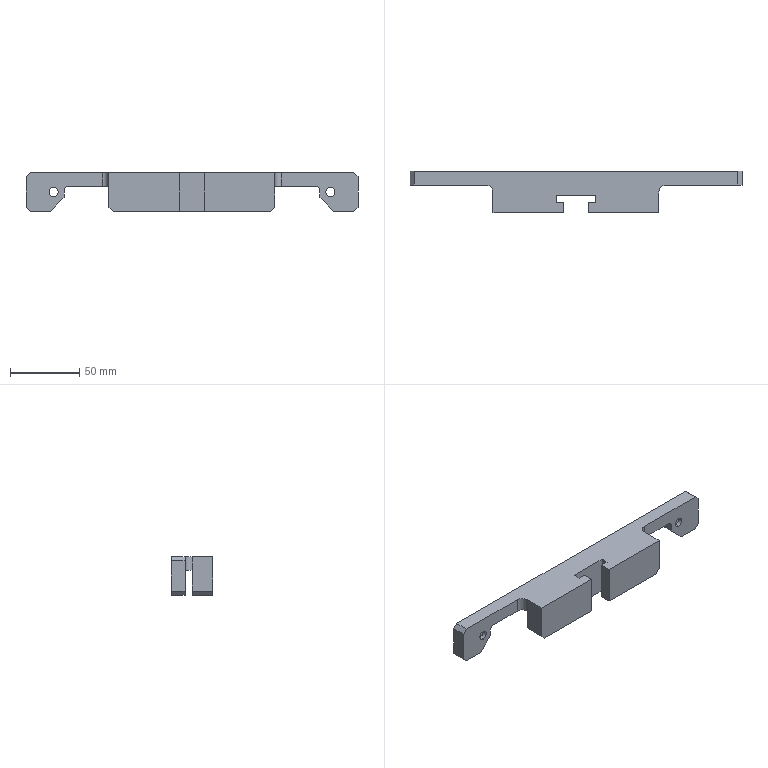Part | SolidWorks | features BaseBody 1 | 1 solid | 46 faces | box 240 x 30 x 28 mm | volume 79875 mm3 | plane 34 | cylinder 12 | commonest cylinder face diameters 6.6 x4 11 x4 6 x2 10 x2
STEP:
#1=CARTESIAN_POINT('',(-100.,8.2,8.5));
#2=VERTEX_POINT('',#1);
#3=CARTESIAN_POINT('',(-100.,8.2,19.5));
#4=VERTEX_POINT('',#3);
#5=CARTESIAN_POINT('',(-100.,8.2,14.));
#6=DIRECTION('',(0.,1.,0.));
#7=DIRECTION('',(0.,0.,1.));
#8=AXIS2_PLACEMENT_3D('',#5,#6,#7);
#9=CIRCLE('',#8,5.5);
#10=EDGE_CURVE('',#2,#4,#9,.T.);
#11=ORIENTED_EDGE('',*,*,#10,.F.);
#12=CARTESIAN_POINT('',(-100.,15.,8.5));
#13=VERTEX_POINT('',#12);
#14=CARTESIAN_POINT('',(-100.,15.,8.5));
#15=DIRECTION('',(0.,1.,0.));
#16=VECTOR('',#15,1000.);
#17=LINE('',#14,#16);
#18=EDGE_CURVE('',#2,#13,#17,.T.);
#19=ORIENTED_EDGE('',*,*,#18,.T.);
#20=CARTESIAN_POINT('',(-100.,15.,19.5));
#21=VERTEX_POINT('',#20);
#22=CARTESIAN_POINT('',(-100.,15.,14.));
#23=DIRECTION('',(0.,1.,0.));
#24=DIRECTION('',(0.,0.,1.));
#25=AXIS2_PLACEMENT_3D('',#22,#23,#24);
#26=CIRCLE('',#25,5.5);
#27=EDGE_CURVE('',#13,#21,#26,.T.);
#28=ORIENTED_EDGE('',*,*,#27,.T.);
#29=CARTESIAN_POINT('',(-100.,15.,19.5));
#30=DIRECTION('',(0.,1.,0.));
#31=VECTOR('',#30,1000.);
#32=LINE('',#29,#31);
#33=EDGE_CURVE('',#4,#21,#32,.T.);
#34=ORIENTED_EDGE('',*,*,#33,.F.);
#35=EDGE_LOOP('',(#11,#19,#28,#34));
#36=FACE_OUTER_BOUND('',#35,.T.);
#37=CARTESIAN_POINT('',(-100.,15.,14.));
#38=DIRECTION('',(0.,1.,0.));
#39=DIRECTION('',(0.,0.,1.));
#40=AXIS2_PLACEMENT_3D('',#37,#38,#39);
#41=CYLINDRICAL_SURFACE('',#40,5.5);
#42=ADVANCED_FACE('',(#36),#41,.F.);
#43=CARTESIAN_POINT('',(-100.,5.,10.7));
#44=VERTEX_POINT('',#43);
#45=CARTESIAN_POINT('',(-100.,5.,17.3));
#46=VERTEX_POINT('',#45);
#47=CARTESIAN_POINT('',(-100.,5.,14.));
#48=DIRECTION('',(0.,1.,0.));
#49=DIRECTION('',(0.,0.,1.));
#50=AXIS2_PLACEMENT_3D('',#47,#48,#49);
#51=CIRCLE('',#50,3.3);
#52=EDGE_CURVE('',#44,#46,#51,.T.);
#53=ORIENTED_EDGE('',*,*,#52,.F.);
#54=CARTESIAN_POINT('',(-100.,8.2,10.7));
#55=VERTEX_POINT('',#54);
#56=CARTESIAN_POINT('',(-100.,15.,10.7));
#57=DIRECTION('',(0.,1.,0.));
#58=VECTOR('',#57,1000.);
#59=LINE('',#56,#58);
#60=EDGE_CURVE('',#44,#55,#59,.T.);
#61=ORIENTED_EDGE('',*,*,#60,.T.);
#62=CARTESIAN_POINT('',(-100.,8.2,17.3));
#63=VERTEX_POINT('',#62);
#64=CARTESIAN_POINT('',(-100.,8.2,14.));
#65=DIRECTION('',(0.,1.,0.));
#66=DIRECTION('',(0.,0.,1.));
#67=AXIS2_PLACEMENT_3D('',#64,#65,#66);
#68=CIRCLE('',#67,3.3);
#69=EDGE_CURVE('',#55,#63,#68,.T.);
#70=ORIENTED_EDGE('',*,*,#69,.T.);
#71=CARTESIAN_POINT('',(-100.,15.,17.3));
#72=DIRECTION('',(0.,1.,0.));
#73=VECTOR('',#72,1000.);
#74=LINE('',#71,#73);
#75=EDGE_CURVE('',#46,#63,#74,.T.);
#76=ORIENTED_EDGE('',*,*,#75,.F.);
#77=EDGE_LOOP('',(#53,#61,#70,#76));
#78=FACE_OUTER_BOUND('',#77,.T.);
#79=CARTESIAN_POINT('',(-100.,15.,14.));
#80=DIRECTION('',(0.,1.,0.));
#81=DIRECTION('',(0.,0.,1.));
#82=AXIS2_PLACEMENT_3D('',#79,#80,#81);
#83=CYLINDRICAL_SURFACE('',#82,3.3);
#84=ADVANCED_FACE('',(#78),#83,.F.);
#85=CARTESIAN_POINT('',(100.,8.2,8.5));
#86=VERTEX_POINT('',#85);
#87=CARTESIAN_POINT('',(100.,8.2,19.5));
#88=VERTEX_POINT('',#87);
#89=CARTESIAN_POINT('',(100.,8.2,14.));
#90=DIRECTION('',(0.,1.,0.));
#91=DIRECTION('',(0.,0.,1.));
#92=AXIS2_PLACEMENT_3D('',#89,#90,#91);
#93=CIRCLE('',#92,5.5);
#94=EDGE_CURVE('',#86,#88,#93,.T.);
#95=ORIENTED_EDGE('',*,*,#94,.F.);
#96=CARTESIAN_POINT('',(100.,15.,8.5));
#97=VERTEX_POINT('',#96);
#98=CARTESIAN_POINT('',(100.,15.,8.5));
#99=DIRECTION('',(0.,1.,0.));
#100=VECTOR('',#99,1000.);
#101=LINE('',#98,#100);
#102=EDGE_CURVE('',#86,#97,#101,.T.);
#103=ORIENTED_EDGE('',*,*,#102,.T.);
#104=CARTESIAN_POINT('',(100.,15.,19.5));
#105=VERTEX_POINT('',#104);
#106=CARTESIAN_POINT('',(100.,15.,14.));
#107=DIRECTION('',(0.,1.,0.));
#108=DIRECTION('',(0.,0.,1.));
#109=AXIS2_PLACEMENT_3D('',#106,#107,#108);
#110=CIRCLE('',#109,5.5);
#111=EDGE_CURVE('',#97,#105,#110,.T.);
#112=ORIENTED_EDGE('',*,*,#111,.T.);
#113=CARTESIAN_POINT('',(100.,15.,19.5));
#114=DIRECTION('',(0.,1.,0.));
#115=VECTOR('',#114,1000.);
#116=LINE('',#113,#115);
#117=EDGE_CURVE('',#88,#105,#116,.T.);
#118=ORIENTED_EDGE('',*,*,#117,.F.);
#119=EDGE_LOOP('',(#95,#103,#112,#118));
#120=FACE_OUTER_BOUND('',#119,.T.);
#121=CARTESIAN_POINT('',(100.,15.,14.));
#122=DIRECTION('',(0.,1.,0.));
#123=DIRECTION('',(0.,0.,1.));
#124=AXIS2_PLACEMENT_3D('',#121,#122,#123);
#125=CYLINDRICAL_SURFACE('',#124,5.5);
#126=ADVANCED_FACE('',(#120),#125,.F.);
#127=CARTESIAN_POINT('',(100.,5.,10.7));
#128=VERTEX_POINT('',#127);
#129=CARTESIAN_POINT('',(100.,5.,17.3));
#130=VERTEX_POINT('',#129);
#131=CARTESIAN_POINT('',(100.,5.,14.));
#132=DIRECTION('',(0.,1.,0.));
#133=DIRECTION('',(-1.,0.,0.));
#134=AXIS2_PLACEMENT_3D('',#131,#132,#133);
#135=CIRCLE('',#134,3.3);
#136=EDGE_CURVE('',#128,#130,#135,.T.);
#137=ORIENTED_EDGE('',*,*,#136,.F.);
#138=CARTESIAN_POINT('',(100.,8.2,10.7));
#139=VERTEX_POINT('',#138);
#140=CARTESIAN_POINT('',(100.,15.,10.7));
#141=DIRECTION('',(0.,1.,0.));
#142=VECTOR('',#141,1000.);
#143=LINE('',#140,#142);
#144=EDGE_CURVE('',#128,#139,#143,.T.);
#145=ORIENTED_EDGE('',*,*,#144,.T.);
#146=CARTESIAN_POINT('',(100.,8.2,17.3));
#147=VERTEX_POINT('',#146);
#148=CARTESIAN_POINT('',(100.,8.2,14.));
#149=DIRECTION('',(0.,1.,0.));
#150=DIRECTION('',(0.,0.,1.));
#151=AXIS2_PLACEMENT_3D('',#148,#149,#150);
#152=CIRCLE('',#151,3.3);
#153=EDGE_CURVE('',#139,#147,#152,.T.);
#154=ORIENTED_EDGE('',*,*,#153,.T.);
#155=CARTESIAN_POINT('',(100.,15.,17.3));
#156=DIRECTION('',(0.,1.,0.));
#157=VECTOR('',#156,1000.);
#158=LINE('',#155,#157);
#159=EDGE_CURVE('',#130,#147,#158,.T.);
#160=ORIENTED_EDGE('',*,*,#159,.F.);
#161=EDGE_LOOP('',(#137,#145,#154,#160));
#162=FACE_OUTER_BOUND('',#161,.T.);
#163=CARTESIAN_POINT('',(100.,15.,14.));
#164=DIRECTION('',(0.,1.,0.));
#165=DIRECTION('',(0.,0.,1.));
#166=AXIS2_PLACEMENT_3D('',#163,#164,#165);
#167=CYLINDRICAL_SURFACE('',#166,3.3);
#168=ADVANCED_FACE('',(#162),#167,.F.);
#169=CARTESIAN_POINT('',(117.,15.,0.));
#170=VERTEX_POINT('',#169);
#171=CARTESIAN_POINT('',(102.5,15.,0.));
#172=VERTEX_POINT('',#171);
#173=CARTESIAN_POINT('',(120.,15.,0.));
#174=DIRECTION('',(-1.,0.,0.));
#175=VECTOR('',#174,1000.);
#176=LINE('',#173,#175);
#177=EDGE_CURVE('',#170,#172,#176,.T.);
#178=ORIENTED_EDGE('',*,*,#177,.F.);
#179=CARTESIAN_POINT('',(117.,5.,0.));
#180=VERTEX_POINT('',#179);
#181=CARTESIAN_POINT('',(117.,0.,0.));
#182=DIRECTION('',(0.,-1.,0.));
#183=VECTOR('',#182,1000.);
#184=LINE('',#181,#183);
#185=EDGE_CURVE('',#170,#180,#184,.T.);
#186=ORIENTED_EDGE('',*,*,#185,.T.);
#187=CARTESIAN_POINT('',(102.5,5.,0.));
#188=VERTEX_POINT('',#187);
#189=CARTESIAN_POINT('',(120.,5.,0.));
#190=DIRECTION('',(-1.,0.,0.));
#191=VECTOR('',#190,1000.);
#192=LINE('',#189,#191);
#193=EDGE_CURVE('',#180,#188,#192,.T.);
#194=ORIENTED_EDGE('',*,*,#193,.T.);
#195=CARTESIAN_POINT('',(102.5,0.,0.));
#196=DIRECTION('',(0.,1.,0.));
#197=VECTOR('',#196,1000.);
#198=LINE('',#195,#197);
#199=EDGE_CURVE('',#188,#172,#198,.T.);
#200=ORIENTED_EDGE('',*,*,#199,.T.);
#201=EDGE_LOOP('',(#178,#186,#194,#200));
#202=FACE_OUTER_BOUND('',#201,.T.);
#203=CARTESIAN_POINT('',(0.,0.,0.));
#204=DIRECTION('',(0.,0.,1.));
#205=DIRECTION('',(1.,0.,0.));
#206=AXIS2_PLACEMENT_3D('',#203,#204,#205);
#207=PLANE('',#206);
#208=ADVANCED_FACE('',(#202),#207,.F.);
#209=CARTESIAN_POINT('',(-102.5,5.,0.));
#210=VERTEX_POINT('',#209);
#211=CARTESIAN_POINT('',(-117.,5.,0.));
#212=VERTEX_POINT('',#211);
#213=CARTESIAN_POINT('',(-120.,5.,0.));
#214=DIRECTION('',(-1.,0.,0.));
#215=VECTOR('',#214,1000.);
#216=LINE('',#213,#215);
#217=EDGE_CURVE('',#210,#212,#216,.T.);
#218=ORIENTED_EDGE('',*,*,#217,.T.);
#219=CARTESIAN_POINT('',(-117.,15.,0.));
#220=VERTEX_POINT('',#219);
#221=CARTESIAN_POINT('',(-117.,0.,0.));
#222=DIRECTION('',(0.,1.,0.));
#223=VECTOR('',#222,1000.);
#224=LINE('',#221,#223);
#225=EDGE_CURVE('',#212,#220,#224,.T.);
#226=ORIENTED_EDGE('',*,*,#225,.T.);
#227=CARTESIAN_POINT('',(-102.5,15.,0.));
#228=VERTEX_POINT('',#227);
#229=CARTESIAN_POINT('',(120.,15.,0.));
#230=DIRECTION('',(-1.,0.,0.));
#231=VECTOR('',#230,1000.);
#232=LINE('',#229,#231);
#233=EDGE_CURVE('',#228,#220,#232,.T.);
#234=ORIENTED_EDGE('',*,*,#233,.F.);
#235=CARTESIAN_POINT('',(-102.5,0.,0.));
#236=DIRECTION('',(0.,-1.,0.));
#237=VECTOR('',#236,1000.);
#238=LINE('',#235,#237);
#239=EDGE_CURVE('',#228,#210,#238,.T.);
#240=ORIENTED_EDGE('',*,*,#239,.T.);
#241=EDGE_LOOP('',(#218,#226,#234,#240));
#242=FACE_OUTER_BOUND('',#241,.T.);
#243=CARTESIAN_POINT('',(0.,0.,0.));
#244=DIRECTION('',(0.,0.,1.));
#245=DIRECTION('',(1.,0.,0.));
#246=AXIS2_PLACEMENT_3D('',#243,#244,#245);
#247=PLANE('',#246);
#248=ADVANCED_FACE('',(#242),#247,.F.);
#249=CARTESIAN_POINT('',(8.75,-15.,0.));
#250=VERTEX_POINT('',#249);
#251=CARTESIAN_POINT('',(57.,-15.,0.));
#252=VERTEX_POINT('',#251);
#253=CARTESIAN_POINT('',(120.,-15.,0.));
#254=DIRECTION('',(1.,0.,0.));
#255=VECTOR('',#254,1000.);
#256=LINE('',#253,#255);
#257=EDGE_CURVE('',#250,#252,#256,.T.);
#258=ORIENTED_EDGE('',*,*,#257,.T.);
#259=CARTESIAN_POINT('',(60.,-15.,3.));
#260=VERTEX_POINT('',#259);
#261=CARTESIAN_POINT('',(57.,-15.,0.));
#262=DIRECTION('',(0.7071,0.,0.7071));
#263=VECTOR('',#262,1000.);
#264=LINE('',#261,#263);
#265=EDGE_CURVE('',#252,#260,#264,.T.);
#266=ORIENTED_EDGE('',*,*,#265,.T.);
#267=CARTESIAN_POINT('',(60.,-15.,28.));
#268=VERTEX_POINT('',#267);
#269=CARTESIAN_POINT('',(60.,-15.,0.));
#270=DIRECTION('',(0.,0.,1.));
#271=VECTOR('',#270,1000.);
#272=LINE('',#269,#271);
#273=EDGE_CURVE('',#260,#268,#272,.T.);
#274=ORIENTED_EDGE('',*,*,#273,.T.);
#275=CARTESIAN_POINT('',(8.75,-15.,28.));
#276=VERTEX_POINT('',#275);
#277=CARTESIAN_POINT('',(120.,-15.,28.));
#278=DIRECTION('',(1.,0.,0.));
#279=VECTOR('',#278,1000.);
#280=LINE('',#277,#279);
#281=EDGE_CURVE('',#276,#268,#280,.T.);
#282=ORIENTED_EDGE('',*,*,#281,.F.);
#283=CARTESIAN_POINT('',(8.75,-15.,28.));
#284=DIRECTION('',(0.,0.,-1.));
#285=VECTOR('',#284,1000.);
#286=LINE('',#283,#285);
#287=EDGE_CURVE('',#276,#250,#286,.T.);
#288=ORIENTED_EDGE('',*,*,#287,.T.);
#289=EDGE_LOOP('',(#258,#266,#274,#282,#288));
#290=FACE_OUTER_BOUND('',#289,.T.);
#291=CARTESIAN_POINT('',(120.,-15.,28.));
#292=DIRECTION('',(0.,1.,0.));
#293=DIRECTION('',(-1.,0.,0.));
#294=AXIS2_PLACEMENT_3D('',#291,#292,#293);
#295=PLANE('',#294);
#296=ADVANCED_FACE('',(#290),#295,.F.);
#297=CARTESIAN_POINT('',(-120.,5.,3.));
#298=VERTEX_POINT('',#297);
#299=CARTESIAN_POINT('',(-120.,5.,25.));
#300=VERTEX_POINT('',#299);
#301=CARTESIAN_POINT('',(-120.,5.,0.));
#302=DIRECTION('',(0.,0.,1.));
#303=VECTOR('',#302,1000.);
#304=LINE('',#301,#303);
#305=EDGE_CURVE('',#298,#300,#304,.T.);
#306=ORIENTED_EDGE('',*,*,#305,.T.);
#307=CARTESIAN_POINT('',(-120.,15.,25.));
#308=VERTEX_POINT('',#307);
#309=CARTESIAN_POINT('',(-120.,15.,25.));
#310=DIRECTION('',(0.,1.,0.));
#311=VECTOR('',#310,1000.);
#312=LINE('',#309,#311);
#313=EDGE_CURVE('',#300,#308,#312,.T.);
#314=ORIENTED_EDGE('',*,*,#313,.T.);
#315=CARTESIAN_POINT('',(-120.,15.,3.));
#316=VERTEX_POINT('',#315);
#317=CARTESIAN_POINT('',(-120.,15.,28.));
#318=DIRECTION('',(0.,0.,-1.));
#319=VECTOR('',#318,1000.);
#320=LINE('',#317,#319);
#321=EDGE_CURVE('',#308,#316,#320,.T.);
#322=ORIENTED_EDGE('',*,*,#321,.T.);
#323=CARTESIAN_POINT('',(-120.,-15.,3.));
#324=DIRECTION('',(0.,-1.,0.));
#325=VECTOR('',#324,1000.);
#326=LINE('',#323,#325);
#327=EDGE_CURVE('',#316,#298,#326,.T.);
#328=ORIENTED_EDGE('',*,*,#327,.T.);
#329=EDGE_LOOP('',(#306,#314,#322,#328));
#330=FACE_OUTER_BOUND('',#329,.T.);
#331=CARTESIAN_POINT('',(-120.,-15.,28.));
#332=DIRECTION('',(1.,0.,0.));
#333=DIRECTION('',(0.,0.,-1.));
#334=AXIS2_PLACEMENT_3D('',#331,#332,#333);
#335=PLANE('',#334);
#336=ADVANCED_FACE('',(#330),#335,.F.);
#337=CARTESIAN_POINT('',(-60.,-15.,3.));
#338=VERTEX_POINT('',#337);
#339=CARTESIAN_POINT('',(-60.,-15.,28.));
#340=VERTEX_POINT('',#339);
#341=CARTESIAN_POINT('',(-60.,-15.,0.));
#342=DIRECTION('',(0.,0.,1.));
#343=VECTOR('',#342,1000.);
#344=LINE('',#341,#343);
#345=EDGE_CURVE('',#338,#340,#344,.T.);
#346=ORIENTED_EDGE('',*,*,#345,.F.);
#347=CARTESIAN_POINT('',(-57.,-15.,0.));
#348=VERTEX_POINT('',#347);
#349=CARTESIAN_POINT('',(-57.,-15.,0.));
#350=DIRECTION('',(0.7071,0.,-0.7071));
#351=VECTOR('',#350,1000.);
#352=LINE('',#349,#351);
#353=EDGE_CURVE('',#338,#348,#352,.T.);
#354=ORIENTED_EDGE('',*,*,#353,.T.);
#355=CARTESIAN_POINT('',(-8.75,-15.,0.));
#356=VERTEX_POINT('',#355);
#357=CARTESIAN_POINT('',(120.,-15.,0.));
#358=DIRECTION('',(1.,0.,0.));
#359=VECTOR('',#358,1000.);
#360=LINE('',#357,#359);
#361=EDGE_CURVE('',#348,#356,#360,.T.);
#362=ORIENTED_EDGE('',*,*,#361,.T.);
#363=CARTESIAN_POINT('',(-8.75,-15.,28.));
#364=VERTEX_POINT('',#363);
#365=CARTESIAN_POINT('',(-8.75,-15.,28.));
#366=DIRECTION('',(0.,0.,1.));
#367=VECTOR('',#366,1000.);
#368=LINE('',#365,#367);
#369=EDGE_CURVE('',#356,#364,#368,.T.);
#370=ORIENTED_EDGE('',*,*,#369,.T.);
#371=CARTESIAN_POINT('',(120.,-15.,28.));
#372=DIRECTION('',(1.,0.,0.));
#373=VECTOR('',#372,1000.);
#374=LINE('',#371,#373);
#375=EDGE_CURVE('',#340,#364,#374,.T.);
#376=ORIENTED_EDGE('',*,*,#375,.F.);
#377=EDGE_LOOP('',(#346,#354,#362,#370,#376));
#378=FACE_OUTER_BOUND('',#377,.T.);
#379=CARTESIAN_POINT('',(120.,-15.,28.));
#380=DIRECTION('',(0.,1.,0.));
#381=DIRECTION('',(-1.,0.,0.));
#382=AXIS2_PLACEMENT_3D('',#379,#380,#381);
#383=PLANE('',#382);
#384=ADVANCED_FACE('',(#378),#383,.F.);
#385=CARTESIAN_POINT('',(120.,5.,3.));
#386=VERTEX_POINT('',#385);
#387=CARTESIAN_POINT('',(120.,5.,25.));
#388=VERTEX_POINT('',#387);
#389=CARTESIAN_POINT('',(120.,5.,0.));
#390=DIRECTION('',(0.,0.,1.));
#391=VECTOR('',#390,1000.);
#392=LINE('',#389,#391);
#393=EDGE_CURVE('',#386,#388,#392,.T.);
#394=ORIENTED_EDGE('',*,*,#393,.F.);
#395=CARTESIAN_POINT('',(120.,15.,3.));
#396=VERTEX_POINT('',#395);
#397=CARTESIAN_POINT('',(120.,-15.,3.));
#398=DIRECTION('',(0.,1.,0.));
#399=VECTOR('',#398,1000.);
#400=LINE('',#397,#399);
#401=EDGE_CURVE('',#386,#396,#400,.T.);
#402=ORIENTED_EDGE('',*,*,#401,.T.);
#403=CARTESIAN_POINT('',(120.,15.,25.));
#404=VERTEX_POINT('',#403);
#405=CARTESIAN_POINT('',(120.,15.,28.));
#406=DIRECTION('',(0.,0.,-1.));
#407=VECTOR('',#406,1000.);
#408=LINE('',#405,#407);
#409=EDGE_CURVE('',#404,#396,#408,.T.);
#410=ORIENTED_EDGE('',*,*,#409,.F.);
#411=CARTESIAN_POINT('',(120.,5.,25.));
#412=DIRECTION('',(0.,-1.,0.));
#413=VECTOR('',#412,1000.);
#414=LINE('',#411,#413);
#415=EDGE_CURVE('',#404,#388,#414,.T.);
#416=ORIENTED_EDGE('',*,*,#415,.T.);
#417=EDGE_LOOP('',(#394,#402,#410,#416));
#418=FACE_OUTER_BOUND('',#417,.T.);
#419=CARTESIAN_POINT('',(120.,-15.,28.));
#420=DIRECTION('',(-1.,0.,0.));
#421=DIRECTION('',(0.,0.,1.));
#422=AXIS2_PLACEMENT_3D('',#419,#420,#421);
#423=PLANE('',#422);
#424=ADVANCED_FACE('',(#418),#423,.F.);
#425=CARTESIAN_POINT('',(-100.,15.,14.));
#426=DIRECTION('',(0.,1.,0.));
#427=DIRECTION('',(0.,0.,1.));
#428=AXIS2_PLACEMENT_3D('',#425,#426,#427);
#429=CIRCLE('',#428,5.5);
#430=EDGE_CURVE('',#21,#13,#429,.T.);
#431=ORIENTED_EDGE('',*,*,#430,.F.);
#432=ORIENTED_EDGE('',*,*,#27,.F.);
#433=EDGE_LOOP('',(#431,#432));
#434=FACE_BOUND('',#433,.T.);
#435=CARTESIAN_POINT('',(100.,15.,14.));
#436=DIRECTION('',(0.,1.,0.));
#437=DIRECTION('',(0.,0.,1.));
#438=AXIS2_PLACEMENT_3D('',#435,#436,#437);
#439=CIRCLE('',#438,5.5);
#440=EDGE_CURVE('',#105,#97,#439,.T.);
#441=ORIENTED_EDGE('',*,*,#440,.F.);
#442=ORIENTED_EDGE('',*,*,#111,.F.);
#443=EDGE_LOOP('',(#441,#442));
#444=FACE_BOUND('',#443,.T.);
#445=ORIENTED_EDGE('',*,*,#321,.F.);
#446=CARTESIAN_POINT('',(-117.,15.,28.));
#447=VERTEX_POINT('',#446);
#448=CARTESIAN_POINT('',(-117.,15.,28.));
#449=DIRECTION('',(0.7071,0.,0.7071));
#450=VECTOR('',#449,1000.);
#451=LINE('',#448,#450);
#452=EDGE_CURVE('',#308,#447,#451,.T.);
#453=ORIENTED_EDGE('',*,*,#452,.T.);
#454=CARTESIAN_POINT('',(117.,15.,28.));
#455=VERTEX_POINT('',#454);
#456=CARTESIAN_POINT('',(120.,15.,28.));
#457=DIRECTION('',(-1.,0.,0.));
#458=VECTOR('',#457,1000.);
#459=LINE('',#456,#458);
#460=EDGE_CURVE('',#455,#447,#459,.T.);
#461=ORIENTED_EDGE('',*,*,#460,.F.);
#462=CARTESIAN_POINT('',(117.,15.,28.));
#463=DIRECTION('',(0.7071,0.,-0.7071));
#464=VECTOR('',#463,1000.);
#465=LINE('',#462,#464);
#466=EDGE_CURVE('',#455,#404,#465,.T.);
#467=ORIENTED_EDGE('',*,*,#466,.T.);
#468=ORIENTED_EDGE('',*,*,#409,.T.);
#469=CARTESIAN_POINT('',(120.,15.,3.));
#470=DIRECTION('',(-0.7071,0.,-0.7071));
#471=VECTOR('',#470,1000.);
#472=LINE('',#469,#471);
#473=EDGE_CURVE('',#396,#170,#472,.T.);
#474=ORIENTED_EDGE('',*,*,#473,.T.);
#475=ORIENTED_EDGE('',*,*,#177,.T.);
#476=CARTESIAN_POINT('',(92.5,15.,10.));
#477=VERTEX_POINT('',#476);
#478=CARTESIAN_POINT('',(92.5,15.,10.));
#479=DIRECTION('',(-0.7071,0.,0.7071));
#480=VECTOR('',#479,1000.);
#481=LINE('',#478,#480);
#482=EDGE_CURVE('',#172,#477,#481,.T.);
#483=ORIENTED_EDGE('',*,*,#482,.T.);
#484=CARTESIAN_POINT('',(92.5,15.,15.));
#485=VERTEX_POINT('',#484);
#486=CARTESIAN_POINT('',(92.5,15.,18.));
#487=DIRECTION('',(0.,0.,-1.));
#488=VECTOR('',#487,1000.);
#489=LINE('',#486,#488);
#490=EDGE_CURVE('',#485,#477,#489,.T.);
#491=ORIENTED_EDGE('',*,*,#490,.F.);
#492=CARTESIAN_POINT('',(89.5,15.,18.));
#493=VERTEX_POINT('',#492);
#494=CARTESIAN_POINT('',(89.5,15.,15.));
#495=DIRECTION('',(0.,-1.,0.));
#496=DIRECTION('',(1.,0.,0.));
#497=AXIS2_PLACEMENT_3D('',#494,#495,#496);
#498=CIRCLE('',#497,3.);
#499=EDGE_CURVE('',#485,#493,#498,.T.);
#500=ORIENTED_EDGE('',*,*,#499,.T.);
#501=CARTESIAN_POINT('',(-89.5,15.,18.));
#502=VERTEX_POINT('',#501);
#503=CARTESIAN_POINT('',(-92.5,15.,18.));
#504=DIRECTION('',(1.,0.,0.));
#505=VECTOR('',#504,1000.);
#506=LINE('',#503,#505);
#507=EDGE_CURVE('',#502,#493,#506,.T.);
#508=ORIENTED_EDGE('',*,*,#507,.F.);
#509=CARTESIAN_POINT('',(-92.5,15.,15.));
#510=VERTEX_POINT('',#509);
#511=CARTESIAN_POINT('',(-89.5,15.,15.));
#512=DIRECTION('',(0.,-1.,0.));
#513=DIRECTION('',(1.,0.,0.));
#514=AXIS2_PLACEMENT_3D('',#511,#512,#513);
#515=CIRCLE('',#514,3.);
#516=EDGE_CURVE('',#502,#510,#515,.T.);
#517=ORIENTED_EDGE('',*,*,#516,.T.);
#518=CARTESIAN_POINT('',(-92.5,15.,10.));
#519=VERTEX_POINT('',#518);
#520=CARTESIAN_POINT('',(-92.5,15.,18.));
#521=DIRECTION('',(0.,0.,-1.));
#522=VECTOR('',#521,1000.);
#523=LINE('',#520,#522);
#524=EDGE_CURVE('',#510,#519,#523,.T.);
#525=ORIENTED_EDGE('',*,*,#524,.T.);
#526=CARTESIAN_POINT('',(-92.5,15.,10.));
#527=DIRECTION('',(-0.7071,0.,-0.7071));
#528=VECTOR('',#527,1000.);
#529=LINE('',#526,#528);
#530=EDGE_CURVE('',#519,#228,#529,.T.);
#531=ORIENTED_EDGE('',*,*,#530,.T.);
#532=ORIENTED_EDGE('',*,*,#233,.T.);
#533=CARTESIAN_POINT('',(-120.,15.,3.));
#534=DIRECTION('',(-0.7071,0.,0.7071));
#535=VECTOR('',#534,1000.);
#536=LINE('',#533,#535);
#537=EDGE_CURVE('',#220,#316,#536,.T.);
#538=ORIENTED_EDGE('',*,*,#537,.T.);
#539=EDGE_LOOP('',(#445,#453,#461,#467,#468,#474,#475,#483,#491,#500,#508,#517,#525,#531,#532,#538));
#540=FACE_OUTER_BOUND('',#539,.T.);
#541=CARTESIAN_POINT('',(120.,15.,28.));
#542=DIRECTION('',(0.,-1.,0.));
#543=DIRECTION('',(1.,0.,0.));
#544=AXIS2_PLACEMENT_3D('',#541,#542,#543);
#545=PLANE('',#544);
#546=ADVANCED_FACE('',(#434,#444,#540),#545,.F.);
#547=ORIENTED_EDGE('',*,*,#460,.T.);
#548=CARTESIAN_POINT('',(-117.,5.,28.));
#549=VERTEX_POINT('',#548);
#550=CARTESIAN_POINT('',(-117.,5.,28.));
#551=DIRECTION('',(0.,-1.,0.));
#552=VECTOR('',#551,1000.);
#553=LINE('',#550,#552);
#554=EDGE_CURVE('',#447,#549,#553,.T.);
#555=ORIENTED_EDGE('',*,*,#554,.T.);
#556=CARTESIAN_POINT('',(-65.,5.,28.));
#557=VERTEX_POINT('',#556);
#558=CARTESIAN_POINT('',(-120.,5.,28.));
#559=DIRECTION('',(-1.,0.,0.));
#560=VECTOR('',#559,1000.);
#561=LINE('',#558,#560);
#562=EDGE_CURVE('',#557,#549,#561,.T.);
#563=ORIENTED_EDGE('',*,*,#562,.F.);
#564=CARTESIAN_POINT('',(-60.,0.,28.));
#565=VERTEX_POINT('',#564);
#566=CARTESIAN_POINT('',(-65.,0.,28.));
#567=DIRECTION('',(0.,0.,-1.));
#568=DIRECTION('',(1.,0.,0.));
#569=AXIS2_PLACEMENT_3D('',#566,#567,#568);
#570=CIRCLE('',#569,5.);
#571=EDGE_CURVE('',#557,#565,#570,.T.);
#572=ORIENTED_EDGE('',*,*,#571,.T.);
#573=CARTESIAN_POINT('',(-60.,-15.,28.));
#574=DIRECTION('',(0.,1.,0.));
#575=VECTOR('',#574,1000.);
#576=LINE('',#573,#575);
#577=EDGE_CURVE('',#340,#565,#576,.T.);
#578=ORIENTED_EDGE('',*,*,#577,.F.);
#579=ORIENTED_EDGE('',*,*,#375,.T.);
#580=CARTESIAN_POINT('',(-8.75,-7.5,28.));
#581=VERTEX_POINT('',#580);
#582=CARTESIAN_POINT('',(-8.75,-22.5,28.));
#583=DIRECTION('',(0.,-1.,0.));
#584=VECTOR('',#583,1000.);
#585=LINE('',#582,#584);
#586=EDGE_CURVE('',#581,#364,#585,.T.);
#587=ORIENTED_EDGE('',*,*,#586,.F.);
#588=CARTESIAN_POINT('',(-14.25,-7.5,28.));
#589=VERTEX_POINT('',#588);
#590=CARTESIAN_POINT('',(14.25,-7.5,28.));
#591=DIRECTION('',(1.,0.,0.));
#592=VECTOR('',#591,1000.);
#593=LINE('',#590,#592);
#594=EDGE_CURVE('',#589,#581,#593,.T.);
#595=ORIENTED_EDGE('',*,*,#594,.F.);
#596=CARTESIAN_POINT('',(-14.25,-2.4,28.));
#597=VERTEX_POINT('',#596);
#598=CARTESIAN_POINT('',(-14.25,-2.4,28.));
#599=DIRECTION('',(0.,-1.,0.));
#600=VECTOR('',#599,1000.);
#601=LINE('',#598,#600);
#602=EDGE_CURVE('',#597,#589,#601,.T.);
#603=ORIENTED_EDGE('',*,*,#602,.F.);
#604=CARTESIAN_POINT('',(14.25,-2.4,28.));
#605=VERTEX_POINT('',#604);
#606=CARTESIAN_POINT('',(14.25,-2.4,28.));
#607=DIRECTION('',(-1.,0.,0.));
#608=VECTOR('',#607,1000.);
#609=LINE('',#606,#608);
#610=EDGE_CURVE('',#605,#597,#609,.T.);
#611=ORIENTED_EDGE('',*,*,#610,.F.);
#612=CARTESIAN_POINT('',(14.25,-7.5,28.));
#613=VERTEX_POINT('',#612);
#614=CARTESIAN_POINT('',(14.25,-2.4,28.));
#615=DIRECTION('',(0.,1.,0.));
#616=VECTOR('',#615,1000.);
#617=LINE('',#614,#616);
#618=EDGE_CURVE('',#613,#605,#617,.T.);
#619=ORIENTED_EDGE('',*,*,#618,.F.);
#620=CARTESIAN_POINT('',(8.75,-7.5,28.));
#621=VERTEX_POINT('',#620);
#622=CARTESIAN_POINT('',(14.25,-7.5,28.));
#623=DIRECTION('',(1.,0.,0.));
#624=VECTOR('',#623,1000.);
#625=LINE('',#622,#624);
#626=EDGE_CURVE('',#621,#613,#625,.T.);
#627=ORIENTED_EDGE('',*,*,#626,.F.);
#628=CARTESIAN_POINT('',(8.75,-22.5,28.));
#629=DIRECTION('',(0.,1.,0.));
#630=VECTOR('',#629,1000.);
#631=LINE('',#628,#630);
#632=EDGE_CURVE('',#276,#621,#631,.T.);
#633=ORIENTED_EDGE('',*,*,#632,.F.);
#634=ORIENTED_EDGE('',*,*,#281,.T.);
#635=CARTESIAN_POINT('',(60.,0.,28.));
#636=VERTEX_POINT('',#635);
#637=CARTESIAN_POINT('',(60.,-15.,28.));
#638=DIRECTION('',(0.,-1.,0.));
#639=VECTOR('',#638,1000.);
#640=LINE('',#637,#639);
#641=EDGE_CURVE('',#636,#268,#640,.T.);
#642=ORIENTED_EDGE('',*,*,#641,.F.);
#643=CARTESIAN_POINT('',(65.,5.,28.));
#644=VERTEX_POINT('',#643);
#645=CARTESIAN_POINT('',(65.,0.,28.));
#646=DIRECTION('',(0.,0.,-1.));
#647=DIRECTION('',(1.,0.,0.));
#648=AXIS2_PLACEMENT_3D('',#645,#646,#647);
#649=CIRCLE('',#648,5.);
#650=EDGE_CURVE('',#636,#644,#649,.T.);
#651=ORIENTED_EDGE('',*,*,#650,.T.);
#652=CARTESIAN_POINT('',(117.,5.,28.));
#653=VERTEX_POINT('',#652);
#654=CARTESIAN_POINT('',(120.,5.,28.));
#655=DIRECTION('',(-1.,0.,0.));
#656=VECTOR('',#655,1000.);
#657=LINE('',#654,#656);
#658=EDGE_CURVE('',#653,#644,#657,.T.);
#659=ORIENTED_EDGE('',*,*,#658,.F.);
#660=CARTESIAN_POINT('',(117.,15.,28.));
#661=DIRECTION('',(0.,1.,0.));
#662=VECTOR('',#661,1000.);
#663=LINE('',#660,#662);
#664=EDGE_CURVE('',#653,#455,#663,.T.);
#665=ORIENTED_EDGE('',*,*,#664,.T.);
#666=EDGE_LOOP('',(#547,#555,#563,#572,#578,#579,#587,#595,#603,#611,#619,#627,#633,#634,#642,#651,#659,#665));
#667=FACE_OUTER_BOUND('',#666,.T.);
#668=CARTESIAN_POINT('',(0.,0.,28.));
#669=DIRECTION('',(0.,0.,1.));
#670=DIRECTION('',(1.,0.,0.));
#671=AXIS2_PLACEMENT_3D('',#668,#669,#670);
#672=PLANE('',#671);
#673=ADVANCED_FACE('',(#667),#672,.T.);
#674=ORIENTED_EDGE('',*,*,#361,.F.);
#675=CARTESIAN_POINT('',(-57.,0.,0.));
#676=VERTEX_POINT('',#675);
#677=CARTESIAN_POINT('',(-57.,0.,0.));
#678=DIRECTION('',(0.,1.,0.));
#679=VECTOR('',#678,1000.);
#680=LINE('',#677,#679);
#681=EDGE_CURVE('',#348,#676,#680,.T.);
#682=ORIENTED_EDGE('',*,*,#681,.T.);
#683=CARTESIAN_POINT('',(57.,0.,0.));
#684=VERTEX_POINT('',#683);
#685=CARTESIAN_POINT('',(-92.5,0.,0.));
#686=DIRECTION('',(-1.,0.,0.));
#687=VECTOR('',#686,1000.);
#688=LINE('',#685,#687);
#689=EDGE_CURVE('',#684,#676,#688,.T.);
#690=ORIENTED_EDGE('',*,*,#689,.F.);
#691=CARTESIAN_POINT('',(57.,0.,0.));
#692=DIRECTION('',(0.,-1.,0.));
#693=VECTOR('',#692,1000.);
#694=LINE('',#691,#693);
#695=EDGE_CURVE('',#684,#252,#694,.T.);
#696=ORIENTED_EDGE('',*,*,#695,.T.);
#697=ORIENTED_EDGE('',*,*,#257,.F.);
#698=CARTESIAN_POINT('',(8.75,-7.5,0.));
#699=VERTEX_POINT('',#698);
#700=CARTESIAN_POINT('',(8.75,0.,0.));
#701=DIRECTION('',(0.,1.,0.));
#702=VECTOR('',#701,1000.);
#703=LINE('',#700,#702);
#704=EDGE_CURVE('',#250,#699,#703,.T.);
#705=ORIENTED_EDGE('',*,*,#704,.T.);
#706=CARTESIAN_POINT('',(14.25,-7.5,0.));
#707=VERTEX_POINT('',#706);
#708=CARTESIAN_POINT('',(14.25,-7.5,0.));
#709=DIRECTION('',(1.,0.,0.));
#710=VECTOR('',#709,1000.);
#711=LINE('',#708,#710);
#712=EDGE_CURVE('',#699,#707,#711,.T.);
#713=ORIENTED_EDGE('',*,*,#712,.T.);
#714=CARTESIAN_POINT('',(14.25,-2.4,0.));
#715=VERTEX_POINT('',#714);
#716=CARTESIAN_POINT('',(14.25,-2.4,0.));
#717=DIRECTION('',(0.,1.,0.));
#718=VECTOR('',#717,1000.);
#719=LINE('',#716,#718);
#720=EDGE_CURVE('',#707,#715,#719,.T.);
#721=ORIENTED_EDGE('',*,*,#720,.T.);
#722=CARTESIAN_POINT('',(-14.25,-2.4,0.));
#723=VERTEX_POINT('',#722);
#724=CARTESIAN_POINT('',(14.25,-2.4,0.));
#725=DIRECTION('',(-1.,0.,0.));
#726=VECTOR('',#725,1000.);
#727=LINE('',#724,#726);
#728=EDGE_CURVE('',#715,#723,#727,.T.);
#729=ORIENTED_EDGE('',*,*,#728,.T.);
#730=CARTESIAN_POINT('',(-14.25,-7.5,0.));
#731=VERTEX_POINT('',#730);
#732=CARTESIAN_POINT('',(-14.25,-2.4,0.));
#733=DIRECTION('',(0.,-1.,0.));
#734=VECTOR('',#733,1000.);
#735=LINE('',#732,#734);
#736=EDGE_CURVE('',#723,#731,#735,.T.);
#737=ORIENTED_EDGE('',*,*,#736,.T.);
#738=CARTESIAN_POINT('',(-8.75,-7.5,0.));
#739=VERTEX_POINT('',#738);
#740=CARTESIAN_POINT('',(14.25,-7.5,0.));
#741=DIRECTION('',(1.,0.,0.));
#742=VECTOR('',#741,1000.);
#743=LINE('',#740,#742);
#744=EDGE_CURVE('',#731,#739,#743,.T.);
#745=ORIENTED_EDGE('',*,*,#744,.T.);
#746=CARTESIAN_POINT('',(-8.75,-22.5,0.));
#747=DIRECTION('',(0.,-1.,0.));
#748=VECTOR('',#747,1000.);
#749=LINE('',#746,#748);
#750=EDGE_CURVE('',#739,#356,#749,.T.);
#751=ORIENTED_EDGE('',*,*,#750,.T.);
#752=EDGE_LOOP('',(#674,#682,#690,#696,#697,#705,#713,#721,#729,#737,#745,#751));
#753=FACE_OUTER_BOUND('',#752,.T.);
#754=CARTESIAN_POINT('',(0.,0.,0.));
#755=DIRECTION('',(0.,0.,1.));
#756=DIRECTION('',(1.,0.,0.));
#757=AXIS2_PLACEMENT_3D('',#754,#755,#756);
#758=PLANE('',#757);
#759=ADVANCED_FACE('',(#753),#758,.F.);
#760=CARTESIAN_POINT('',(-100.,5.,14.));
#761=DIRECTION('',(0.,1.,0.));
#762=DIRECTION('',(0.,0.,1.));
#763=AXIS2_PLACEMENT_3D('',#760,#761,#762);
#764=CIRCLE('',#763,3.3);
#765=EDGE_CURVE('',#46,#44,#764,.T.);
#766=ORIENTED_EDGE('',*,*,#765,.T.);
#767=ORIENTED_EDGE('',*,*,#52,.T.);
#768=EDGE_LOOP('',(#766,#767));
#769=FACE_BOUND('',#768,.T.);
#770=ORIENTED_EDGE('',*,*,#562,.T.);
#771=CARTESIAN_POINT('',(-117.,5.,28.));
#772=DIRECTION('',(-0.7071,0.,-0.7071));
#773=VECTOR('',#772,1000.);
#774=LINE('',#771,#773);
#775=EDGE_CURVE('',#549,#300,#774,.T.);
#776=ORIENTED_EDGE('',*,*,#775,.T.);
#777=ORIENTED_EDGE('',*,*,#305,.F.);
#778=CARTESIAN_POINT('',(-120.,5.,3.));
#779=DIRECTION('',(0.7071,0.,-0.7071));
#780=VECTOR('',#779,1000.);
#781=LINE('',#778,#780);
#782=EDGE_CURVE('',#298,#212,#781,.T.);
#783=ORIENTED_EDGE('',*,*,#782,.T.);
#784=ORIENTED_EDGE('',*,*,#217,.F.);
#785=CARTESIAN_POINT('',(-92.5,5.,10.));
#786=VERTEX_POINT('',#785);
#787=CARTESIAN_POINT('',(-92.5,5.,10.));
#788=DIRECTION('',(0.7071,0.,0.7071));
#789=VECTOR('',#788,1000.);
#790=LINE('',#787,#789);
#791=EDGE_CURVE('',#210,#786,#790,.T.);
#792=ORIENTED_EDGE('',*,*,#791,.T.);
#793=CARTESIAN_POINT('',(-92.5,5.,15.));
#794=VERTEX_POINT('',#793);
#795=CARTESIAN_POINT('',(-92.5,5.,0.));
#796=DIRECTION('',(0.,0.,1.));
#797=VECTOR('',#796,1000.);
#798=LINE('',#795,#797);
#799=EDGE_CURVE('',#786,#794,#798,.T.);
#800=ORIENTED_EDGE('',*,*,#799,.T.);
#801=CARTESIAN_POINT('',(-89.5,5.,18.));
#802=VERTEX_POINT('',#801);
#803=CARTESIAN_POINT('',(-89.5,5.,15.));
#804=DIRECTION('',(0.,1.,0.));
#805=DIRECTION('',(0.,0.,1.));
#806=AXIS2_PLACEMENT_3D('',#803,#804,#805);
#807=CIRCLE('',#806,3.);
#808=EDGE_CURVE('',#794,#802,#807,.T.);
#809=ORIENTED_EDGE('',*,*,#808,.T.);
#810=CARTESIAN_POINT('',(-65.,5.,18.));
#811=VERTEX_POINT('',#810);
#812=CARTESIAN_POINT('',(-120.,5.,18.));
#813=DIRECTION('',(1.,0.,0.));
#814=VECTOR('',#813,1000.);
#815=LINE('',#812,#814);
#816=EDGE_CURVE('',#802,#811,#815,.T.);
#817=ORIENTED_EDGE('',*,*,#816,.T.);
#818=CARTESIAN_POINT('',(-65.,5.,28.));
#819=DIRECTION('',(0.,0.,1.));
#820=VECTOR('',#819,1000.);
#821=LINE('',#818,#820);
#822=EDGE_CURVE('',#811,#557,#821,.T.);
#823=ORIENTED_EDGE('',*,*,#822,.T.);
#824=EDGE_LOOP('',(#770,#776,#777,#783,#784,#792,#800,#809,#817,#823));
#825=FACE_OUTER_BOUND('',#824,.T.);
#826=CARTESIAN_POINT('',(-120.,5.,0.));
#827=DIRECTION('',(0.,1.,0.));
#828=DIRECTION('',(0.,0.,1.));
#829=AXIS2_PLACEMENT_3D('',#826,#827,#828);
#830=PLANE('',#829);
#831=ADVANCED_FACE('',(#769,#825),#830,.F.);
#832=CARTESIAN_POINT('',(-60.,0.,18.));
#833=VERTEX_POINT('',#832);
#834=CARTESIAN_POINT('',(-60.,0.,3.));
#835=VERTEX_POINT('',#834);
#836=CARTESIAN_POINT('',(-60.,0.,0.));
#837=DIRECTION('',(0.,0.,-1.));
#838=VECTOR('',#837,1000.);
#839=LINE('',#836,#838);
#840=EDGE_CURVE('',#833,#835,#839,.T.);
#841=ORIENTED_EDGE('',*,*,#840,.T.);
#842=CARTESIAN_POINT('',(-60.,-15.,3.));
#843=DIRECTION('',(0.,-1.,0.));
#844=VECTOR('',#843,1000.);
#845=LINE('',#842,#844);
#846=EDGE_CURVE('',#835,#338,#845,.T.);
#847=ORIENTED_EDGE('',*,*,#846,.T.);
#848=ORIENTED_EDGE('',*,*,#345,.T.);
#849=ORIENTED_EDGE('',*,*,#577,.T.);
#850=CARTESIAN_POINT('',(-60.,0.,0.));
#851=DIRECTION('',(0.,0.,-1.));
#852=VECTOR('',#851,1000.);
#853=LINE('',#850,#852);
#854=EDGE_CURVE('',#565,#833,#853,.T.);
#855=ORIENTED_EDGE('',*,*,#854,.T.);
#856=EDGE_LOOP('',(#841,#847,#848,#849,#855));
#857=FACE_OUTER_BOUND('',#856,.T.);
#858=CARTESIAN_POINT('',(-60.,-15.,0.));
#859=DIRECTION('',(1.,0.,0.));
#860=DIRECTION('',(0.,0.,-1.));
#861=AXIS2_PLACEMENT_3D('',#858,#859,#860);
#862=PLANE('',#861);
#863=ADVANCED_FACE('',(#857),#862,.F.);
#864=ORIENTED_EDGE('',*,*,#273,.F.);
#865=CARTESIAN_POINT('',(60.,0.,3.));
#866=VERTEX_POINT('',#865);
#867=CARTESIAN_POINT('',(60.,-15.,3.));
#868=DIRECTION('',(0.,1.,0.));
#869=VECTOR('',#868,1000.);
#870=LINE('',#867,#869);
#871=EDGE_CURVE('',#260,#866,#870,.T.);
#872=ORIENTED_EDGE('',*,*,#871,.T.);
#873=CARTESIAN_POINT('',(60.,0.,18.));
#874=VERTEX_POINT('',#873);
#875=CARTESIAN_POINT('',(60.,0.,28.));
#876=DIRECTION('',(0.,0.,1.));
#877=VECTOR('',#876,1000.);
#878=LINE('',#875,#877);
#879=EDGE_CURVE('',#866,#874,#878,.T.);
#880=ORIENTED_EDGE('',*,*,#879,.T.);
#881=CARTESIAN_POINT('',(60.,0.,28.));
#882=DIRECTION('',(0.,0.,1.));
#883=VECTOR('',#882,1000.);
#884=LINE('',#881,#883);
#885=EDGE_CURVE('',#874,#636,#884,.T.);
#886=ORIENTED_EDGE('',*,*,#885,.T.);
#887=ORIENTED_EDGE('',*,*,#641,.T.);
#888=EDGE_LOOP('',(#864,#872,#880,#886,#887));
#889=FACE_OUTER_BOUND('',#888,.T.);
#890=CARTESIAN_POINT('',(60.,-15.,0.));
#891=DIRECTION('',(-1.,0.,0.));
#892=DIRECTION('',(0.,0.,1.));
#893=AXIS2_PLACEMENT_3D('',#890,#891,#892);
#894=PLANE('',#893);
#895=ADVANCED_FACE('',(#889),#894,.F.);
#896=CARTESIAN_POINT('',(100.,5.,14.));
#897=DIRECTION('',(0.,1.,0.));
#898=DIRECTION('',(-1.,0.,0.));
#899=AXIS2_PLACEMENT_3D('',#896,#897,#898);
#900=CIRCLE('',#899,3.3);
#901=EDGE_CURVE('',#130,#128,#900,.T.);
#902=ORIENTED_EDGE('',*,*,#901,.T.);
#903=ORIENTED_EDGE('',*,*,#136,.T.);
#904=EDGE_LOOP('',(#902,#903));
#905=FACE_BOUND('',#904,.T.);
#906=ORIENTED_EDGE('',*,*,#193,.F.);
#907=CARTESIAN_POINT('',(120.,5.,3.));
#908=DIRECTION('',(0.7071,0.,0.7071));
#909=VECTOR('',#908,1000.);
#910=LINE('',#907,#909);
#911=EDGE_CURVE('',#180,#386,#910,.T.);
#912=ORIENTED_EDGE('',*,*,#911,.T.);
#913=ORIENTED_EDGE('',*,*,#393,.T.);
#914=CARTESIAN_POINT('',(117.,5.,28.));
#915=DIRECTION('',(-0.7071,0.,0.7071));
#916=VECTOR('',#915,1000.);
#917=LINE('',#914,#916);
#918=EDGE_CURVE('',#388,#653,#917,.T.);
#919=ORIENTED_EDGE('',*,*,#918,.T.);
#920=ORIENTED_EDGE('',*,*,#658,.T.);
#921=CARTESIAN_POINT('',(65.,5.,18.));
#922=VERTEX_POINT('',#921);
#923=CARTESIAN_POINT('',(65.,5.,0.));
#924=DIRECTION('',(0.,0.,-1.));
#925=VECTOR('',#924,1000.);
#926=LINE('',#923,#925);
#927=EDGE_CURVE('',#644,#922,#926,.T.);
#928=ORIENTED_EDGE('',*,*,#927,.T.);
#929=CARTESIAN_POINT('',(89.5,5.,18.));
#930=VERTEX_POINT('',#929);
#931=CARTESIAN_POINT('',(120.,5.,18.));
#932=DIRECTION('',(1.,0.,0.));
#933=VECTOR('',#932,1000.);
#934=LINE('',#931,#933);
#935=EDGE_CURVE('',#922,#930,#934,.T.);
#936=ORIENTED_EDGE('',*,*,#935,.T.);
#937=CARTESIAN_POINT('',(92.5,5.,15.));
#938=VERTEX_POINT('',#937);
#939=CARTESIAN_POINT('',(89.5,5.,15.));
#940=DIRECTION('',(0.,1.,0.));
#941=DIRECTION('',(-1.,0.,0.));
#942=AXIS2_PLACEMENT_3D('',#939,#940,#941);
#943=CIRCLE('',#942,3.);
#944=EDGE_CURVE('',#930,#938,#943,.T.);
#945=ORIENTED_EDGE('',*,*,#944,.T.);
#946=CARTESIAN_POINT('',(92.5,5.,10.));
#947=VERTEX_POINT('',#946);
#948=CARTESIAN_POINT('',(92.5,5.,0.));
#949=DIRECTION('',(0.,0.,-1.));
#950=VECTOR('',#949,1000.);
#951=LINE('',#948,#950);
#952=EDGE_CURVE('',#938,#947,#951,.T.);
#953=ORIENTED_EDGE('',*,*,#952,.T.);
#954=CARTESIAN_POINT('',(92.5,5.,10.));
#955=DIRECTION('',(0.7071,0.,-0.7071));
#956=VECTOR('',#955,1000.);
#957=LINE('',#954,#956);
#958=EDGE_CURVE('',#947,#188,#957,.T.);
#959=ORIENTED_EDGE('',*,*,#958,.T.);
#960=EDGE_LOOP('',(#906,#912,#913,#919,#920,#928,#936,#945,#953,#959));
#961=FACE_OUTER_BOUND('',#960,.T.);
#962=CARTESIAN_POINT('',(120.,5.,0.));
#963=DIRECTION('',(0.,1.,0.));
#964=DIRECTION('',(-1.,0.,0.));
#965=AXIS2_PLACEMENT_3D('',#962,#963,#964);
#966=PLANE('',#965);
#967=ADVANCED_FACE('',(#905,#961),#966,.F.);
#968=ORIENTED_EDGE('',*,*,#632,.T.);
#969=CARTESIAN_POINT('',(8.75,-7.5,0.));
#970=DIRECTION('',(0.,0.,1.));
#971=VECTOR('',#970,1000.);
#972=LINE('',#969,#971);
#973=EDGE_CURVE('',#699,#621,#972,.T.);
#974=ORIENTED_EDGE('',*,*,#973,.F.);
#975=ORIENTED_EDGE('',*,*,#704,.F.);
#976=ORIENTED_EDGE('',*,*,#287,.F.);
#977=EDGE_LOOP('',(#968,#974,#975,#976));
#978=FACE_OUTER_BOUND('',#977,.T.);
#979=CARTESIAN_POINT('',(8.75,-22.5,0.));
#980=DIRECTION('',(1.,0.,0.));
#981=DIRECTION('',(0.,0.,-1.));
#982=AXIS2_PLACEMENT_3D('',#979,#980,#981);
#983=PLANE('',#982);
#984=ADVANCED_FACE('',(#978),#983,.F.);
#985=ORIENTED_EDGE('',*,*,#750,.F.);
#986=CARTESIAN_POINT('',(-8.75,-7.5,0.));
#987=DIRECTION('',(0.,0.,1.));
#988=VECTOR('',#987,1000.);
#989=LINE('',#986,#988);
#990=EDGE_CURVE('',#739,#581,#989,.T.);
#991=ORIENTED_EDGE('',*,*,#990,.T.);
#992=ORIENTED_EDGE('',*,*,#586,.T.);
#993=ORIENTED_EDGE('',*,*,#369,.F.);
#994=EDGE_LOOP('',(#985,#991,#992,#993));
#995=FACE_OUTER_BOUND('',#994,.T.);
#996=CARTESIAN_POINT('',(-8.75,-22.5,0.));
#997=DIRECTION('',(-1.,0.,0.));
#998=DIRECTION('',(0.,0.,1.));
#999=AXIS2_PLACEMENT_3D('',#996,#997,#998);
#1000=PLANE('',#999);
#1001=ADVANCED_FACE('',(#995),#1000,.F.);
#1002=ORIENTED_EDGE('',*,*,#626,.T.);
#1003=CARTESIAN_POINT('',(14.25,-7.5,0.));
#1004=DIRECTION('',(0.,0.,1.));
#1005=VECTOR('',#1004,1000.);
#1006=LINE('',#1003,#1005);
#1007=EDGE_CURVE('',#707,#613,#1006,.T.);
#1008=ORIENTED_EDGE('',*,*,#1007,.F.);
#1009=ORIENTED_EDGE('',*,*,#712,.F.);
#1010=ORIENTED_EDGE('',*,*,#973,.T.);
#1011=EDGE_LOOP('',(#1002,#1008,#1009,#1010));
#1012=FACE_OUTER_BOUND('',#1011,.T.);
#1013=CARTESIAN_POINT('',(14.25,-7.5,0.));
#1014=DIRECTION('',(0.,-1.,0.));
#1015=DIRECTION('',(1.,0.,0.));
#1016=AXIS2_PLACEMENT_3D('',#1013,#1014,#1015);
#1017=PLANE('',#1016);
#1018=ADVANCED_FACE('',(#1012),#1017,.F.);
#1019=ORIENTED_EDGE('',*,*,#744,.F.);
#1020=CARTESIAN_POINT('',(-14.25,-7.5,0.));
#1021=DIRECTION('',(0.,0.,1.));
#1022=VECTOR('',#1021,1000.);
#1023=LINE('',#1020,#1022);
#1024=EDGE_CURVE('',#731,#589,#1023,.T.);
#1025=ORIENTED_EDGE('',*,*,#1024,.T.);
#1026=ORIENTED_EDGE('',*,*,#594,.T.);
#1027=ORIENTED_EDGE('',*,*,#990,.F.);
#1028=EDGE_LOOP('',(#1019,#1025,#1026,#1027));
#1029=FACE_OUTER_BOUND('',#1028,.T.);
#1030=CARTESIAN_POINT('',(14.25,-7.5,0.));
#1031=DIRECTION('',(0.,-1.,0.));
#1032=DIRECTION('',(1.,0.,0.));
#1033=AXIS2_PLACEMENT_3D('',#1030,#1031,#1032);
#1034=PLANE('',#1033);
#1035=ADVANCED_FACE('',(#1029),#1034,.F.);
#1036=ORIENTED_EDGE('',*,*,#618,.T.);
#1037=CARTESIAN_POINT('',(14.25,-2.4,0.));
#1038=DIRECTION('',(0.,0.,1.));
#1039=VECTOR('',#1038,1000.);
#1040=LINE('',#1037,#1039);
#1041=EDGE_CURVE('',#715,#605,#1040,.T.);
#1042=ORIENTED_EDGE('',*,*,#1041,.F.);
#1043=ORIENTED_EDGE('',*,*,#720,.F.);
#1044=ORIENTED_EDGE('',*,*,#1007,.T.);
#1045=EDGE_LOOP('',(#1036,#1042,#1043,#1044));
#1046=FACE_OUTER_BOUND('',#1045,.T.);
#1047=CARTESIAN_POINT('',(14.25,-2.4,0.));
#1048=DIRECTION('',(1.,0.,0.));
#1049=DIRECTION('',(0.,0.,-1.));
#1050=AXIS2_PLACEMENT_3D('',#1047,#1048,#1049);
#1051=PLANE('',#1050);
#1052=ADVANCED_FACE('',(#1046),#1051,.F.);
#1053=ORIENTED_EDGE('',*,*,#602,.T.);
#1054=ORIENTED_EDGE('',*,*,#1024,.F.);
#1055=ORIENTED_EDGE('',*,*,#736,.F.);
#1056=CARTESIAN_POINT('',(-14.25,-2.4,0.));
#1057=DIRECTION('',(0.,0.,1.));
#1058=VECTOR('',#1057,1000.);
#1059=LINE('',#1056,#1058);
#1060=EDGE_CURVE('',#723,#597,#1059,.T.);
#1061=ORIENTED_EDGE('',*,*,#1060,.T.);
#1062=EDGE_LOOP('',(#1053,#1054,#1055,#1061));
#1063=FACE_OUTER_BOUND('',#1062,.T.);
#1064=CARTESIAN_POINT('',(-14.25,-2.4,0.));
#1065=DIRECTION('',(-1.,0.,0.));
#1066=DIRECTION('',(0.,-1.,0.));
#1067=AXIS2_PLACEMENT_3D('',#1064,#1065,#1066);
#1068=PLANE('',#1067);
#1069=ADVANCED_FACE('',(#1063),#1068,.F.);
#1070=ORIENTED_EDGE('',*,*,#610,.T.);
#1071=ORIENTED_EDGE('',*,*,#1060,.F.);
#1072=ORIENTED_EDGE('',*,*,#728,.F.);
#1073=ORIENTED_EDGE('',*,*,#1041,.T.);
#1074=EDGE_LOOP('',(#1070,#1071,#1072,#1073));
#1075=FACE_OUTER_BOUND('',#1074,.T.);
#1076=CARTESIAN_POINT('',(14.25,-2.4,0.));
#1077=DIRECTION('',(0.,1.,0.));
#1078=DIRECTION('',(-1.,0.,0.));
#1079=AXIS2_PLACEMENT_3D('',#1076,#1077,#1078);
#1080=PLANE('',#1079);
#1081=ADVANCED_FACE('',(#1075),#1080,.F.);
#1082=ORIENTED_EDGE('',*,*,#885,.F.);
#1083=CARTESIAN_POINT('',(65.,0.,18.));
#1084=DIRECTION('',(0.,0.,-1.));
#1085=DIRECTION('',(1.,0.,0.));
#1086=AXIS2_PLACEMENT_3D('',#1083,#1084,#1085);
#1087=CIRCLE('',#1086,5.);
#1088=EDGE_CURVE('',#874,#922,#1087,.T.);
#1089=ORIENTED_EDGE('',*,*,#1088,.T.);
#1090=ORIENTED_EDGE('',*,*,#927,.F.);
#1091=ORIENTED_EDGE('',*,*,#650,.F.);
#1092=EDGE_LOOP('',(#1082,#1089,#1090,#1091));
#1093=FACE_OUTER_BOUND('',#1092,.T.);
#1094=CARTESIAN_POINT('',(65.,0.,0.));
#1095=DIRECTION('',(0.,0.,-1.));
#1096=DIRECTION('',(-1.,0.,0.));
#1097=AXIS2_PLACEMENT_3D('',#1094,#1095,#1096);
#1098=CYLINDRICAL_SURFACE('',#1097,5.);
#1099=ADVANCED_FACE('',(#1093),#1098,.F.);
#1100=ORIENTED_EDGE('',*,*,#822,.F.);
#1101=CARTESIAN_POINT('',(-65.,0.,18.));
#1102=DIRECTION('',(0.,0.,-1.));
#1103=DIRECTION('',(1.,0.,0.));
#1104=AXIS2_PLACEMENT_3D('',#1101,#1102,#1103);
#1105=CIRCLE('',#1104,5.);
#1106=EDGE_CURVE('',#811,#833,#1105,.T.);
#1107=ORIENTED_EDGE('',*,*,#1106,.T.);
#1108=ORIENTED_EDGE('',*,*,#854,.F.);
#1109=ORIENTED_EDGE('',*,*,#571,.F.);
#1110=EDGE_LOOP('',(#1100,#1107,#1108,#1109));
#1111=FACE_OUTER_BOUND('',#1110,.T.);
#1112=CARTESIAN_POINT('',(-65.,0.,0.));
#1113=DIRECTION('',(0.,0.,-1.));
#1114=DIRECTION('',(-1.,0.,0.));
#1115=AXIS2_PLACEMENT_3D('',#1112,#1113,#1114);
#1116=CYLINDRICAL_SURFACE('',#1115,5.);
#1117=ADVANCED_FACE('',(#1111),#1116,.F.);
#1118=ORIENTED_EDGE('',*,*,#799,.F.);
#1119=CARTESIAN_POINT('',(-92.5,15.,10.));
#1120=DIRECTION('',(0.,1.,0.));
#1121=VECTOR('',#1120,1000.);
#1122=LINE('',#1119,#1121);
#1123=EDGE_CURVE('',#786,#519,#1122,.T.);
#1124=ORIENTED_EDGE('',*,*,#1123,.T.);
#1125=ORIENTED_EDGE('',*,*,#524,.F.);
#1126=CARTESIAN_POINT('',(-92.5,5.,15.));
#1127=DIRECTION('',(0.,-1.,0.));
#1128=VECTOR('',#1127,1000.);
#1129=LINE('',#1126,#1128);
#1130=EDGE_CURVE('',#510,#794,#1129,.T.);
#1131=ORIENTED_EDGE('',*,*,#1130,.T.);
#1132=EDGE_LOOP('',(#1118,#1124,#1125,#1131));
#1133=FACE_OUTER_BOUND('',#1132,.T.);
#1134=CARTESIAN_POINT('',(-92.5,15.,18.));
#1135=DIRECTION('',(-1.,0.,0.));
#1136=DIRECTION('',(0.,0.,1.));
#1137=AXIS2_PLACEMENT_3D('',#1134,#1135,#1136);
#1138=PLANE('',#1137);
#1139=ADVANCED_FACE('',(#1133),#1138,.F.);
#1140=ORIENTED_EDGE('',*,*,#490,.T.);
#1141=CARTESIAN_POINT('',(92.5,15.,10.));
#1142=DIRECTION('',(0.,-1.,0.));
#1143=VECTOR('',#1142,1000.);
#1144=LINE('',#1141,#1143);
#1145=EDGE_CURVE('',#477,#947,#1144,.T.);
#1146=ORIENTED_EDGE('',*,*,#1145,.T.);
#1147=ORIENTED_EDGE('',*,*,#952,.F.);
#1148=CARTESIAN_POINT('',(92.5,15.,15.));
#1149=DIRECTION('',(0.,1.,0.));
#1150=VECTOR('',#1149,1000.);
#1151=LINE('',#1148,#1150);
#1152=EDGE_CURVE('',#938,#485,#1151,.T.);
#1153=ORIENTED_EDGE('',*,*,#1152,.T.);
#1154=EDGE_LOOP('',(#1140,#1146,#1147,#1153));
#1155=FACE_OUTER_BOUND('',#1154,.T.);
#1156=CARTESIAN_POINT('',(92.5,15.,18.));
#1157=DIRECTION('',(1.,0.,0.));
#1158=DIRECTION('',(0.,0.,-1.));
#1159=AXIS2_PLACEMENT_3D('',#1156,#1157,#1158);
#1160=PLANE('',#1159);
#1161=ADVANCED_FACE('',(#1155),#1160,.F.);
#1162=ORIENTED_EDGE('',*,*,#689,.T.);
#1163=CARTESIAN_POINT('',(-57.,0.,0.));
#1164=DIRECTION('',(-0.7071,0.,0.7071));
#1165=VECTOR('',#1164,1000.);
#1166=LINE('',#1163,#1165);
#1167=EDGE_CURVE('',#676,#835,#1166,.T.);
#1168=ORIENTED_EDGE('',*,*,#1167,.T.);
#1169=ORIENTED_EDGE('',*,*,#840,.F.);
#1170=CARTESIAN_POINT('',(-92.5,0.,18.));
#1171=DIRECTION('',(-1.,0.,0.));
#1172=VECTOR('',#1171,1000.);
#1173=LINE('',#1170,#1172);
#1174=EDGE_CURVE('',#874,#833,#1173,.T.);
#1175=ORIENTED_EDGE('',*,*,#1174,.F.);
#1176=ORIENTED_EDGE('',*,*,#879,.F.);
#1177=CARTESIAN_POINT('',(57.,0.,0.));
#1178=DIRECTION('',(-0.7071,0.,-0.7071));
#1179=VECTOR('',#1178,1000.);
#1180=LINE('',#1177,#1179);
#1181=EDGE_CURVE('',#866,#684,#1180,.T.);
#1182=ORIENTED_EDGE('',*,*,#1181,.T.);
#1183=EDGE_LOOP('',(#1162,#1168,#1169,#1175,#1176,#1182));
#1184=FACE_OUTER_BOUND('',#1183,.T.);
#1185=CARTESIAN_POINT('',(-92.5,0.,18.));
#1186=DIRECTION('',(0.,-1.,0.));
#1187=DIRECTION('',(0.,0.,-1.));
#1188=AXIS2_PLACEMENT_3D('',#1185,#1186,#1187);
#1189=PLANE('',#1188);
#1190=ADVANCED_FACE('',(#1184),#1189,.F.);
#1191=ORIENTED_EDGE('',*,*,#507,.T.);
#1192=CARTESIAN_POINT('',(89.5,5.,18.));
#1193=DIRECTION('',(0.,-1.,0.));
#1194=VECTOR('',#1193,1000.);
#1195=LINE('',#1192,#1194);
#1196=EDGE_CURVE('',#493,#930,#1195,.T.);
#1197=ORIENTED_EDGE('',*,*,#1196,.T.);
#1198=ORIENTED_EDGE('',*,*,#935,.F.);
#1199=ORIENTED_EDGE('',*,*,#1088,.F.);
#1200=ORIENTED_EDGE('',*,*,#1174,.T.);
#1201=ORIENTED_EDGE('',*,*,#1106,.F.);
#1202=ORIENTED_EDGE('',*,*,#816,.F.);
#1203=CARTESIAN_POINT('',(-89.5,15.,18.));
#1204=DIRECTION('',(0.,1.,0.));
#1205=VECTOR('',#1204,1000.);
#1206=LINE('',#1203,#1205);
#1207=EDGE_CURVE('',#802,#502,#1206,.T.);
#1208=ORIENTED_EDGE('',*,*,#1207,.T.);
#1209=EDGE_LOOP('',(#1191,#1197,#1198,#1199,#1200,#1201,#1202,#1208));
#1210=FACE_OUTER_BOUND('',#1209,.T.);
#1211=CARTESIAN_POINT('',(0.,0.,18.));
#1212=DIRECTION('',(0.,0.,1.));
#1213=DIRECTION('',(1.,0.,0.));
#1214=AXIS2_PLACEMENT_3D('',#1211,#1212,#1213);
#1215=PLANE('',#1214);
#1216=ADVANCED_FACE('',(#1210),#1215,.F.);
#1217=ORIENTED_EDGE('',*,*,#499,.F.);
#1218=ORIENTED_EDGE('',*,*,#1152,.F.);
#1219=ORIENTED_EDGE('',*,*,#944,.F.);
#1220=ORIENTED_EDGE('',*,*,#1196,.F.);
#1221=EDGE_LOOP('',(#1217,#1218,#1219,#1220));
#1222=FACE_OUTER_BOUND('',#1221,.T.);
#1223=CARTESIAN_POINT('',(89.5,0.,15.));
#1224=DIRECTION('',(0.,1.,0.));
#1225=DIRECTION('',(0.,0.,1.));
#1226=AXIS2_PLACEMENT_3D('',#1223,#1224,#1225);
#1227=CYLINDRICAL_SURFACE('',#1226,3.);
#1228=ADVANCED_FACE('',(#1222),#1227,.F.);
#1229=ORIENTED_EDGE('',*,*,#808,.F.);
#1230=ORIENTED_EDGE('',*,*,#1130,.F.);
#1231=ORIENTED_EDGE('',*,*,#516,.F.);
#1232=ORIENTED_EDGE('',*,*,#1207,.F.);
#1233=EDGE_LOOP('',(#1229,#1230,#1231,#1232));
#1234=FACE_OUTER_BOUND('',#1233,.T.);
#1235=CARTESIAN_POINT('',(-89.5,0.,15.));
#1236=DIRECTION('',(0.,-1.,0.));
#1237=DIRECTION('',(0.,0.,-1.));
#1238=AXIS2_PLACEMENT_3D('',#1235,#1236,#1237);
#1239=CYLINDRICAL_SURFACE('',#1238,3.);
#1240=ADVANCED_FACE('',(#1234),#1239,.F.);
#1241=ORIENTED_EDGE('',*,*,#482,.F.);
#1242=ORIENTED_EDGE('',*,*,#199,.F.);
#1243=ORIENTED_EDGE('',*,*,#958,.F.);
#1244=ORIENTED_EDGE('',*,*,#1145,.F.);
#1245=EDGE_LOOP('',(#1241,#1242,#1243,#1244));
#1246=FACE_OUTER_BOUND('',#1245,.T.);
#1247=CARTESIAN_POINT('',(92.5,15.,10.));
#1248=DIRECTION('',(0.7071,0.,0.7071));
#1249=DIRECTION('',(0.,-1.,0.));
#1250=AXIS2_PLACEMENT_3D('',#1247,#1248,#1249);
#1251=PLANE('',#1250);
#1252=ADVANCED_FACE('',(#1246),#1251,.F.);
#1253=ORIENTED_EDGE('',*,*,#791,.F.);
#1254=ORIENTED_EDGE('',*,*,#239,.F.);
#1255=ORIENTED_EDGE('',*,*,#530,.F.);
#1256=ORIENTED_EDGE('',*,*,#1123,.F.);
#1257=EDGE_LOOP('',(#1253,#1254,#1255,#1256));
#1258=FACE_OUTER_BOUND('',#1257,.T.);
#1259=CARTESIAN_POINT('',(-92.5,15.,10.));
#1260=DIRECTION('',(-0.7071,0.,0.7071));
#1261=DIRECTION('',(0.,1.,0.));
#1262=AXIS2_PLACEMENT_3D('',#1259,#1260,#1261);
#1263=PLANE('',#1262);
#1264=ADVANCED_FACE('',(#1258),#1263,.F.);
#1265=ORIENTED_EDGE('',*,*,#353,.F.);
#1266=ORIENTED_EDGE('',*,*,#846,.F.);
#1267=ORIENTED_EDGE('',*,*,#1167,.F.);
#1268=ORIENTED_EDGE('',*,*,#681,.F.);
#1269=EDGE_LOOP('',(#1265,#1266,#1267,#1268));
#1270=FACE_OUTER_BOUND('',#1269,.T.);
#1271=CARTESIAN_POINT('',(-57.,0.,0.));
#1272=DIRECTION('',(0.7071,0.,0.7071));
#1273=DIRECTION('',(0.,1.,0.));
#1274=AXIS2_PLACEMENT_3D('',#1271,#1272,#1273);
#1275=PLANE('',#1274);
#1276=ADVANCED_FACE('',(#1270),#1275,.F.);
#1277=ORIENTED_EDGE('',*,*,#1181,.F.);
#1278=ORIENTED_EDGE('',*,*,#871,.F.);
#1279=ORIENTED_EDGE('',*,*,#265,.F.);
#1280=ORIENTED_EDGE('',*,*,#695,.F.);
#1281=EDGE_LOOP('',(#1277,#1278,#1279,#1280));
#1282=FACE_OUTER_BOUND('',#1281,.T.);
#1283=CARTESIAN_POINT('',(57.,0.,0.));
#1284=DIRECTION('',(-0.7071,0.,0.7071));
#1285=DIRECTION('',(0.,-1.,0.));
#1286=AXIS2_PLACEMENT_3D('',#1283,#1284,#1285);
#1287=PLANE('',#1286);
#1288=ADVANCED_FACE('',(#1282),#1287,.F.);
#1289=ORIENTED_EDGE('',*,*,#452,.F.);
#1290=ORIENTED_EDGE('',*,*,#313,.F.);
#1291=ORIENTED_EDGE('',*,*,#775,.F.);
#1292=ORIENTED_EDGE('',*,*,#554,.F.);
#1293=EDGE_LOOP('',(#1289,#1290,#1291,#1292));
#1294=FACE_OUTER_BOUND('',#1293,.T.);
#1295=CARTESIAN_POINT('',(-117.,0.,28.));
#1296=DIRECTION('',(-0.7071,0.,0.7071));
#1297=DIRECTION('',(0.,1.,0.));
#1298=AXIS2_PLACEMENT_3D('',#1295,#1296,#1297);
#1299=PLANE('',#1298);
#1300=ADVANCED_FACE('',(#1294),#1299,.T.);
#1301=ORIENTED_EDGE('',*,*,#537,.F.);
#1302=ORIENTED_EDGE('',*,*,#225,.F.);
#1303=ORIENTED_EDGE('',*,*,#782,.F.);
#1304=ORIENTED_EDGE('',*,*,#327,.F.);
#1305=EDGE_LOOP('',(#1301,#1302,#1303,#1304));
#1306=FACE_OUTER_BOUND('',#1305,.T.);
#1307=CARTESIAN_POINT('',(-120.,-15.,3.));
#1308=DIRECTION('',(0.7071,0.,0.7071));
#1309=DIRECTION('',(0.,-1.,0.));
#1310=AXIS2_PLACEMENT_3D('',#1307,#1308,#1309);
#1311=PLANE('',#1310);
#1312=ADVANCED_FACE('',(#1306),#1311,.F.);
#1313=ORIENTED_EDGE('',*,*,#911,.F.);
#1314=ORIENTED_EDGE('',*,*,#185,.F.);
#1315=ORIENTED_EDGE('',*,*,#473,.F.);
#1316=ORIENTED_EDGE('',*,*,#401,.F.);
#1317=EDGE_LOOP('',(#1313,#1314,#1315,#1316));
#1318=FACE_OUTER_BOUND('',#1317,.T.);
#1319=CARTESIAN_POINT('',(120.,-15.,3.));
#1320=DIRECTION('',(-0.7071,0.,0.7071));
#1321=DIRECTION('',(0.,1.,0.));
#1322=AXIS2_PLACEMENT_3D('',#1319,#1320,#1321);
#1323=PLANE('',#1322);
#1324=ADVANCED_FACE('',(#1318),#1323,.F.);
#1325=ORIENTED_EDGE('',*,*,#918,.F.);
#1326=ORIENTED_EDGE('',*,*,#415,.F.);
#1327=ORIENTED_EDGE('',*,*,#466,.F.);
#1328=ORIENTED_EDGE('',*,*,#664,.F.);
#1329=EDGE_LOOP('',(#1325,#1326,#1327,#1328));
#1330=FACE_OUTER_BOUND('',#1329,.T.);
#1331=CARTESIAN_POINT('',(117.,0.,28.));
#1332=DIRECTION('',(0.7071,0.,0.7071));
#1333=DIRECTION('',(0.,-1.,0.));
#1334=AXIS2_PLACEMENT_3D('',#1331,#1332,#1333);
#1335=PLANE('',#1334);
#1336=ADVANCED_FACE('',(#1330),#1335,.T.);
#1337=ORIENTED_EDGE('',*,*,#144,.F.);
#1338=ORIENTED_EDGE('',*,*,#901,.F.);
#1339=ORIENTED_EDGE('',*,*,#159,.T.);
#1340=CARTESIAN_POINT('',(100.,8.2,14.));
#1341=DIRECTION('',(0.,1.,0.));
#1342=DIRECTION('',(0.,0.,1.));
#1343=AXIS2_PLACEMENT_3D('',#1340,#1341,#1342);
#1344=CIRCLE('',#1343,3.3);
#1345=EDGE_CURVE('',#147,#139,#1344,.T.);
#1346=ORIENTED_EDGE('',*,*,#1345,.T.);
#1347=EDGE_LOOP('',(#1337,#1338,#1339,#1346));
#1348=FACE_OUTER_BOUND('',#1347,.T.);
#1349=CARTESIAN_POINT('',(100.,15.,14.));
#1350=DIRECTION('',(0.,1.,0.));
#1351=DIRECTION('',(0.,0.,1.));
#1352=AXIS2_PLACEMENT_3D('',#1349,#1350,#1351);
#1353=CYLINDRICAL_SURFACE('',#1352,3.3);
#1354=ADVANCED_FACE('',(#1348),#1353,.F.);
#1355=ORIENTED_EDGE('',*,*,#1345,.F.);
#1356=ORIENTED_EDGE('',*,*,#153,.F.);
#1357=EDGE_LOOP('',(#1355,#1356));
#1358=FACE_BOUND('',#1357,.T.);
#1359=CARTESIAN_POINT('',(100.,8.2,14.));
#1360=DIRECTION('',(0.,1.,0.));
#1361=DIRECTION('',(0.,0.,1.));
#1362=AXIS2_PLACEMENT_3D('',#1359,#1360,#1361);
#1363=CIRCLE('',#1362,5.5);
#1364=EDGE_CURVE('',#88,#86,#1363,.T.);
#1365=ORIENTED_EDGE('',*,*,#1364,.T.);
#1366=ORIENTED_EDGE('',*,*,#94,.T.);
#1367=EDGE_LOOP('',(#1365,#1366));
#1368=FACE_OUTER_BOUND('',#1367,.T.);
#1369=CARTESIAN_POINT('',(103.3,8.2,14.));
#1370=DIRECTION('',(0.,-1.,0.));
#1371=DIRECTION('',(0.,0.,-1.));
#1372=AXIS2_PLACEMENT_3D('',#1369,#1370,#1371);
#1373=PLANE('',#1372);
#1374=ADVANCED_FACE('',(#1358,#1368),#1373,.F.);
#1375=ORIENTED_EDGE('',*,*,#102,.F.);
#1376=ORIENTED_EDGE('',*,*,#1364,.F.);
#1377=ORIENTED_EDGE('',*,*,#117,.T.);
#1378=ORIENTED_EDGE('',*,*,#440,.T.);
#1379=EDGE_LOOP('',(#1375,#1376,#1377,#1378));
#1380=FACE_OUTER_BOUND('',#1379,.T.);
#1381=CARTESIAN_POINT('',(100.,15.,14.));
#1382=DIRECTION('',(0.,1.,0.));
#1383=DIRECTION('',(0.,0.,1.));
#1384=AXIS2_PLACEMENT_3D('',#1381,#1382,#1383);
#1385=CYLINDRICAL_SURFACE('',#1384,5.5);
#1386=ADVANCED_FACE('',(#1380),#1385,.F.);
#1387=ORIENTED_EDGE('',*,*,#60,.F.);
#1388=ORIENTED_EDGE('',*,*,#765,.F.);
#1389=ORIENTED_EDGE('',*,*,#75,.T.);
#1390=CARTESIAN_POINT('',(-100.,8.2,14.));
#1391=DIRECTION('',(0.,1.,0.));
#1392=DIRECTION('',(0.,0.,1.));
#1393=AXIS2_PLACEMENT_3D('',#1390,#1391,#1392);
#1394=CIRCLE('',#1393,3.3);
#1395=EDGE_CURVE('',#63,#55,#1394,.T.);
#1396=ORIENTED_EDGE('',*,*,#1395,.T.);
#1397=EDGE_LOOP('',(#1387,#1388,#1389,#1396));
#1398=FACE_OUTER_BOUND('',#1397,.T.);
#1399=CARTESIAN_POINT('',(-100.,15.,14.));
#1400=DIRECTION('',(0.,1.,0.));
#1401=DIRECTION('',(0.,0.,1.));
#1402=AXIS2_PLACEMENT_3D('',#1399,#1400,#1401);
#1403=CYLINDRICAL_SURFACE('',#1402,3.3);
#1404=ADVANCED_FACE('',(#1398),#1403,.F.);
#1405=ORIENTED_EDGE('',*,*,#1395,.F.);
#1406=ORIENTED_EDGE('',*,*,#69,.F.);
#1407=EDGE_LOOP('',(#1405,#1406));
#1408=FACE_BOUND('',#1407,.T.);
#1409=CARTESIAN_POINT('',(-100.,8.2,14.));
#1410=DIRECTION('',(0.,1.,0.));
#1411=DIRECTION('',(0.,0.,1.));
#1412=AXIS2_PLACEMENT_3D('',#1409,#1410,#1411);
#1413=CIRCLE('',#1412,5.5);
#1414=EDGE_CURVE('',#4,#2,#1413,.T.);
#1415=ORIENTED_EDGE('',*,*,#1414,.T.);
#1416=ORIENTED_EDGE('',*,*,#10,.T.);
#1417=EDGE_LOOP('',(#1415,#1416));
#1418=FACE_OUTER_BOUND('',#1417,.T.);
#1419=CARTESIAN_POINT('',(-96.7,8.2,14.));
#1420=DIRECTION('',(0.,-1.,0.));
#1421=DIRECTION('',(0.,0.,-1.));
#1422=AXIS2_PLACEMENT_3D('',#1419,#1420,#1421);
#1423=PLANE('',#1422);
#1424=ADVANCED_FACE('',(#1408,#1418),#1423,.F.);
#1425=ORIENTED_EDGE('',*,*,#18,.F.);
#1426=ORIENTED_EDGE('',*,*,#1414,.F.);
#1427=ORIENTED_EDGE('',*,*,#33,.T.);
#1428=ORIENTED_EDGE('',*,*,#430,.T.);
#1429=EDGE_LOOP('',(#1425,#1426,#1427,#1428));
#1430=FACE_OUTER_BOUND('',#1429,.T.);
#1431=CARTESIAN_POINT('',(-100.,15.,14.));
#1432=DIRECTION('',(0.,1.,0.));
#1433=DIRECTION('',(0.,0.,1.));
#1434=AXIS2_PLACEMENT_3D('',#1431,#1432,#1433);
#1435=CYLINDRICAL_SURFACE('',#1434,5.5);
#1436=ADVANCED_FACE('',(#1430),#1435,.F.);
#1437=CLOSED_SHELL('',(#42,#84,#126,#168,#208,#248,#296,#336,#384,#424,#546,#673,#759,#831,#863,#895,#967,#984,#1001,#1018,#1035,#1052,#1069,#1081,#1099,#1117,#1139,#1161,#1190,#1216,#1228,#1240,#1252,#1264,#1276,#1288,#1300,#1312,#1324,#1336,#1354,#1374,#1386,#1404,#1424,#1436));
#1438=MANIFOLD_SOLID_BREP('',#1437);
#1439=CARTESIAN_POINT('',(0.,0.,0.));
#1440=DIRECTION('',(0.,0.,1.));
#1441=DIRECTION('',(1.,0.,0.));
#1442=AXIS2_PLACEMENT_3D('',#1439,#1440,#1441);
#1443=(LENGTH_UNIT()NAMED_UNIT(*)SI_UNIT(.MILLI.,.METRE.));
#1444=UNCERTAINTY_MEASURE_WITH_UNIT(LENGTH_MEASURE(0.00001),#1443,'','');
#1445=(NAMED_UNIT(*)PLANE_ANGLE_UNIT()SI_UNIT($,.RADIAN.));
#1446=(NAMED_UNIT(*)SI_UNIT($,.STERADIAN.)SOLID_ANGLE_UNIT());
#1447=(GEOMETRIC_REPRESENTATION_CONTEXT(3)GLOBAL_UNCERTAINTY_ASSIGNED_CONTEXT((#1444))GLOBAL_UNIT_ASSIGNED_CONTEXT((#1443,#1445,#1446))REPRESENTATION_CONTEXT('',''));
#1448=ADVANCED_BREP_SHAPE_REPRESENTATION('',(#1438,#1442),#1447);